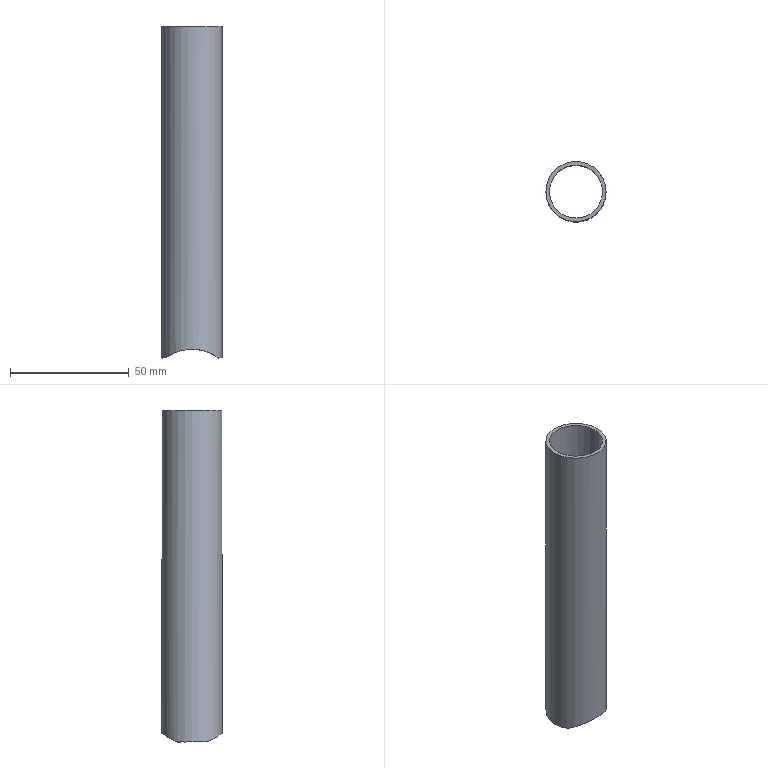Part | STEP file | 6151404 | 1 solid | 7 faces | box 25.4 x 25.4 x 140 mm | volume 15577 mm3 | cylinder 4 | plane 3 | commonest cylinder face diameters 38 x2 22.4 x1 25.4 x1
STEP:
#1=CARTESIAN_POINT('',(11.2,-5.987,-70.));
#2=VERTEX_POINT('',#1);
#3=CARTESIAN_POINT('',(11.2,5.987,-70.));
#4=VERTEX_POINT('',#3);
#5=CARTESIAN_POINT('',(0.,0.,-70.));
#6=DIRECTION('',(0.,0.,1.));
#7=DIRECTION('',(1.,0.,0.));
#8=AXIS2_PLACEMENT_3D('',#5,#6,#7);
#9=CIRCLE('',#8,12.7);
#10=EDGE_CURVE('',#2,#4,#9,.T.);
#11=ORIENTED_EDGE('',*,*,#10,.F.);
#12=CARTESIAN_POINT('',(11.2,0.,-70.));
#13=VERTEX_POINT('',#12);
#14=CARTESIAN_POINT('',(11.2,-30.,-70.));
#15=DIRECTION('',(0.,1.,0.));
#16=VECTOR('',#15,1000.);
#17=LINE('',#14,#16);
#18=EDGE_CURVE('',#2,#13,#17,.T.);
#19=ORIENTED_EDGE('',*,*,#18,.T.);
#20=CARTESIAN_POINT('',(11.2,-30.,-70.));
#21=DIRECTION('',(0.,1.,0.));
#22=VECTOR('',#21,1000.);
#23=LINE('',#20,#22);
#24=EDGE_CURVE('',#13,#4,#23,.T.);
#25=ORIENTED_EDGE('',*,*,#24,.T.);
#26=EDGE_LOOP('',(#11,#19,#25));
#27=FACE_OUTER_BOUND('',#26,.T.);
#28=CARTESIAN_POINT('',(0.,0.,-70.));
#29=DIRECTION('',(0.,0.,1.));
#30=DIRECTION('',(1.,0.,0.));
#31=AXIS2_PLACEMENT_3D('',#28,#29,#30);
#32=PLANE('',#31);
#33=ADVANCED_FACE('',(#27),#32,.F.);
#34=CARTESIAN_POINT('',(12.7,0.,70.));
#35=VERTEX_POINT('',#34);
#36=CARTESIAN_POINT('',(0.,0.,70.));
#37=DIRECTION('',(0.,0.,1.));
#38=DIRECTION('',(1.,0.,0.));
#39=AXIS2_PLACEMENT_3D('',#36,#37,#38);
#40=CIRCLE('',#39,12.7);
#41=EDGE_CURVE('',#35,#35,#40,.T.);
#42=ORIENTED_EDGE('',*,*,#41,.T.);
#43=EDGE_LOOP('',(#42));
#44=FACE_OUTER_BOUND('',#43,.T.);
#45=CARTESIAN_POINT('',(11.2,0.,70.));
#46=VERTEX_POINT('',#45);
#47=CARTESIAN_POINT('',(0.,0.,70.));
#48=DIRECTION('',(0.,0.,1.));
#49=DIRECTION('',(1.,0.,0.));
#50=AXIS2_PLACEMENT_3D('',#47,#48,#49);
#51=CIRCLE('',#50,11.2);
#52=EDGE_CURVE('',#46,#46,#51,.T.);
#53=ORIENTED_EDGE('',*,*,#52,.F.);
#54=EDGE_LOOP('',(#53));
#55=FACE_BOUND('',#54,.T.);
#56=CARTESIAN_POINT('',(0.,0.,70.));
#57=DIRECTION('',(0.,0.,1.));
#58=DIRECTION('',(1.,0.,0.));
#59=AXIS2_PLACEMENT_3D('',#56,#57,#58);
#60=PLANE('',#59);
#61=ADVANCED_FACE('',(#44,#55),#60,.T.);
#62=CARTESIAN_POINT('',(-11.2,5.987,-70.));
#63=VERTEX_POINT('',#62);
#64=CARTESIAN_POINT('',(-11.2,-5.987,-70.));
#65=VERTEX_POINT('',#64);
#66=CARTESIAN_POINT('',(0.,0.,-70.));
#67=DIRECTION('',(0.,0.,1.));
#68=DIRECTION('',(1.,0.,0.));
#69=AXIS2_PLACEMENT_3D('',#66,#67,#68);
#70=CIRCLE('',#69,12.7);
#71=EDGE_CURVE('',#63,#65,#70,.T.);
#72=ORIENTED_EDGE('',*,*,#71,.F.);
#73=CARTESIAN_POINT('',(-11.2,0.,-70.));
#74=VERTEX_POINT('',#73);
#75=CARTESIAN_POINT('',(-11.2,-30.,-70.));
#76=DIRECTION('',(0.,-1.,0.));
#77=VECTOR('',#76,1000.);
#78=LINE('',#75,#77);
#79=EDGE_CURVE('',#63,#74,#78,.T.);
#80=ORIENTED_EDGE('',*,*,#79,.T.);
#81=CARTESIAN_POINT('',(-11.2,-30.,-70.));
#82=DIRECTION('',(0.,-1.,0.));
#83=VECTOR('',#82,1000.);
#84=LINE('',#81,#83);
#85=EDGE_CURVE('',#74,#65,#84,.T.);
#86=ORIENTED_EDGE('',*,*,#85,.T.);
#87=EDGE_LOOP('',(#72,#80,#86));
#88=FACE_OUTER_BOUND('',#87,.T.);
#89=CARTESIAN_POINT('',(0.,0.,-70.));
#90=DIRECTION('',(0.,0.,1.));
#91=DIRECTION('',(1.,0.,0.));
#92=AXIS2_PLACEMENT_3D('',#89,#90,#91);
#93=PLANE('',#92);
#94=ADVANCED_FACE('',(#88),#93,.F.);
#95=ORIENTED_EDGE('',*,*,#41,.F.);
#96=EDGE_LOOP('',(#95));
#97=FACE_OUTER_BOUND('',#96,.T.);
#98=ORIENTED_EDGE('',*,*,#71,.T.);
#99=CARTESIAN_POINT('',(-11.2,-5.987,-70.));
#100=CARTESIAN_POINT('',(-10.665,-6.988,-69.61));
#101=CARTESIAN_POINT('',(-10.02,-7.882,-69.181));
#102=CARTESIAN_POINT('',(-9.072,-8.892,-68.652));
#103=CARTESIAN_POINT('',(-8.875,-9.088,-68.547));
#104=CARTESIAN_POINT('',(-8.467,-9.47,-68.337));
#105=CARTESIAN_POINT('',(-8.255,-9.655,-68.233));
#106=CARTESIAN_POINT('',(-7.604,-10.187,-67.929));
#107=CARTESIAN_POINT('',(-7.149,-10.512,-67.737));
#108=CARTESIAN_POINT('',(-6.192,-11.102,-67.378));
#109=CARTESIAN_POINT('',(-5.692,-11.368,-67.212));
#110=CARTESIAN_POINT('',(-4.639,-11.836,-66.915));
#111=CARTESIAN_POINT('',(-4.085,-12.039,-66.784));
#112=CARTESIAN_POINT('',(-2.962,-12.364,-66.572));
#113=CARTESIAN_POINT('',(-2.388,-12.487,-66.489));
#114=CARTESIAN_POINT('',(-1.215,-12.656,-66.378));
#115=CARTESIAN_POINT('',(-0.6122,-12.699,-66.349));
#116=CARTESIAN_POINT('',(0.5767,-12.701,-66.347));
#117=CARTESIAN_POINT('',(1.167,-12.66,-66.375));
#118=CARTESIAN_POINT('',(2.339,-12.497,-66.483));
#119=CARTESIAN_POINT('',(2.925,-12.373,-66.566));
#120=CARTESIAN_POINT('',(4.053,-12.05,-66.776));
#121=CARTESIAN_POINT('',(4.598,-11.853,-66.905));
#122=CARTESIAN_POINT('',(5.653,-11.387,-67.2));
#123=CARTESIAN_POINT('',(6.165,-11.118,-67.369));
#124=CARTESIAN_POINT('',(7.133,-10.523,-67.73));
#125=CARTESIAN_POINT('',(7.591,-10.197,-67.924));
#126=CARTESIAN_POINT('',(8.458,-9.49,-68.328));
#127=CARTESIAN_POINT('',(8.869,-9.107,-68.539));
#128=CARTESIAN_POINT('',(10.017,-7.887,-69.179));
#129=CARTESIAN_POINT('',(10.665,-6.988,-69.61));
#130=CARTESIAN_POINT('',(11.2,-5.987,-70.));
#131=B_SPLINE_CURVE_WITH_KNOTS('',3,(#99,#100,#101,#102,#103,#104,#105,#106,#107,#108,#109,#110,#111,#112,#113,#114,#115,#116,#117,#118,#119,#120,#121,#122,#123,#124,#125,#126,#127,#128,#129,#130),.UNSPECIFIED.,.F.,.F.,(4,2,2,2,2,2,2,2,2,2,2,2,2,2,2,4),(0.,0.003547,0.004433,0.00532,0.007093,0.008867,0.01064,0.01241,0.01419,0.01596,0.01773,0.01951,0.02128,0.02305,0.02483,0.02837),.UNSPECIFIED.);
#132=EDGE_CURVE('',#65,#2,#131,.T.);
#133=ORIENTED_EDGE('',*,*,#132,.T.);
#134=ORIENTED_EDGE('',*,*,#10,.T.);
#135=CARTESIAN_POINT('',(11.2,5.987,-70.));
#136=CARTESIAN_POINT('',(10.665,6.988,-69.61));
#137=CARTESIAN_POINT('',(10.02,7.882,-69.181));
#138=CARTESIAN_POINT('',(9.072,8.892,-68.652));
#139=CARTESIAN_POINT('',(8.875,9.088,-68.547));
#140=CARTESIAN_POINT('',(8.467,9.47,-68.337));
#141=CARTESIAN_POINT('',(8.255,9.655,-68.233));
#142=CARTESIAN_POINT('',(7.604,10.187,-67.929));
#143=CARTESIAN_POINT('',(7.149,10.512,-67.737));
#144=CARTESIAN_POINT('',(6.192,11.102,-67.378));
#145=CARTESIAN_POINT('',(5.692,11.368,-67.212));
#146=CARTESIAN_POINT('',(4.639,11.836,-66.915));
#147=CARTESIAN_POINT('',(4.085,12.039,-66.784));
#148=CARTESIAN_POINT('',(2.962,12.364,-66.572));
#149=CARTESIAN_POINT('',(2.388,12.487,-66.489));
#150=CARTESIAN_POINT('',(1.215,12.656,-66.378));
#151=CARTESIAN_POINT('',(0.6122,12.699,-66.349));
#152=CARTESIAN_POINT('',(-0.5767,12.701,-66.347));
#153=CARTESIAN_POINT('',(-1.167,12.66,-66.375));
#154=CARTESIAN_POINT('',(-2.339,12.497,-66.483));
#155=CARTESIAN_POINT('',(-2.925,12.373,-66.566));
#156=CARTESIAN_POINT('',(-4.053,12.05,-66.776));
#157=CARTESIAN_POINT('',(-4.598,11.853,-66.905));
#158=CARTESIAN_POINT('',(-5.653,11.387,-67.2));
#159=CARTESIAN_POINT('',(-6.165,11.118,-67.369));
#160=CARTESIAN_POINT('',(-7.133,10.523,-67.73));
#161=CARTESIAN_POINT('',(-7.591,10.197,-67.924));
#162=CARTESIAN_POINT('',(-8.458,9.49,-68.328));
#163=CARTESIAN_POINT('',(-8.869,9.107,-68.539));
#164=CARTESIAN_POINT('',(-10.017,7.887,-69.179));
#165=CARTESIAN_POINT('',(-10.665,6.988,-69.61));
#166=CARTESIAN_POINT('',(-11.2,5.987,-70.));
#167=B_SPLINE_CURVE_WITH_KNOTS('',3,(#135,#136,#137,#138,#139,#140,#141,#142,#143,#144,#145,#146,#147,#148,#149,#150,#151,#152,#153,#154,#155,#156,#157,#158,#159,#160,#161,#162,#163,#164,#165,#166),.UNSPECIFIED.,.F.,.F.,(4,2,2,2,2,2,2,2,2,2,2,2,2,2,2,4),(0.,0.003547,0.004433,0.00532,0.007093,0.008867,0.01064,0.01241,0.01419,0.01596,0.01773,0.01951,0.02128,0.02305,0.02483,0.02837),.UNSPECIFIED.);
#168=EDGE_CURVE('',#4,#63,#167,.T.);
#169=ORIENTED_EDGE('',*,*,#168,.T.);
#170=EDGE_LOOP('',(#98,#133,#134,#169));
#171=FACE_OUTER_BOUND('',#170,.T.);
#172=CARTESIAN_POINT('',(0.,0.,70.));
#173=DIRECTION('',(0.,0.,-1.));
#174=DIRECTION('',(-1.,0.,0.));
#175=AXIS2_PLACEMENT_3D('',#172,#173,#174);
#176=CYLINDRICAL_SURFACE('',#175,12.7);
#177=ADVANCED_FACE('',(#97,#171),#176,.T.);
#178=CARTESIAN_POINT('',(-11.2,0.,-70.));
#179=CARTESIAN_POINT('',(-11.2,-0.7603,-70.));
#180=CARTESIAN_POINT('',(-11.123,-1.503,-69.943));
#181=CARTESIAN_POINT('',(-10.828,-2.956,-69.734));
#182=CARTESIAN_POINT('',(-10.606,-3.673,-69.58));
#183=CARTESIAN_POINT('',(-10.04,-5.016,-69.214));
#184=CARTESIAN_POINT('',(-9.698,-5.65,-69.003));
#185=CARTESIAN_POINT('',(-8.89,-6.851,-68.55));
#186=CARTESIAN_POINT('',(-8.436,-7.401,-68.315));
#187=CARTESIAN_POINT('',(-7.681,-8.159,-67.968));
#188=CARTESIAN_POINT('',(-7.417,-8.4,-67.853));
#189=CARTESIAN_POINT('',(-6.862,-8.859,-67.628));
#190=CARTESIAN_POINT('',(-6.57,-9.077,-67.517));
#191=CARTESIAN_POINT('',(-5.674,-9.683,-67.204));
#192=CARTESIAN_POINT('',(-5.04,-10.029,-67.016));
#193=CARTESIAN_POINT('',(-4.03,-10.456,-66.777));
#194=CARTESIAN_POINT('',(-3.684,-10.584,-66.705));
#195=CARTESIAN_POINT('',(-2.969,-10.806,-66.578));
#196=CARTESIAN_POINT('',(-2.607,-10.899,-66.524));
#197=CARTESIAN_POINT('',(-1.514,-11.122,-66.394));
#198=CARTESIAN_POINT('',(-0.7732,-11.199,-66.349));
#199=CARTESIAN_POINT('',(0.3582,-11.201,-66.348));
#200=CARTESIAN_POINT('',(0.7396,-11.182,-66.359));
#201=CARTESIAN_POINT('',(1.488,-11.107,-66.403));
#202=CARTESIAN_POINT('',(1.857,-11.051,-66.435));
#203=CARTESIAN_POINT('',(2.587,-10.903,-66.521));
#204=CARTESIAN_POINT('',(2.947,-10.812,-66.574));
#205=CARTESIAN_POINT('',(3.66,-10.592,-66.7));
#206=CARTESIAN_POINT('',(4.011,-10.464,-66.773));
#207=CARTESIAN_POINT('',(5.029,-10.035,-67.012));
#208=CARTESIAN_POINT('',(5.667,-9.688,-67.202));
#209=CARTESIAN_POINT('',(6.57,-9.078,-67.517));
#210=CARTESIAN_POINT('',(6.861,-8.86,-67.628));
#211=CARTESIAN_POINT('',(7.415,-8.401,-67.852));
#212=CARTESIAN_POINT('',(7.679,-8.161,-67.967));
#213=CARTESIAN_POINT('',(8.183,-7.655,-68.198));
#214=CARTESIAN_POINT('',(8.423,-7.391,-68.315));
#215=CARTESIAN_POINT('',(8.878,-6.837,-68.548));
#216=CARTESIAN_POINT('',(9.095,-6.546,-68.664));
#217=CARTESIAN_POINT('',(9.697,-5.65,-69.002));
#218=CARTESIAN_POINT('',(10.039,-5.019,-69.213));
#219=CARTESIAN_POINT('',(10.461,-4.017,-69.486));
#220=CARTESIAN_POINT('',(10.587,-3.673,-69.57));
#221=CARTESIAN_POINT('',(10.807,-2.965,-69.72));
#222=CARTESIAN_POINT('',(10.9,-2.601,-69.785));
#223=CARTESIAN_POINT('',(11.123,-1.505,-69.943));
#224=CARTESIAN_POINT('',(11.2,-0.7604,-70.));
#225=CARTESIAN_POINT('',(11.2,0.,-70.));
#226=B_SPLINE_CURVE_WITH_KNOTS('',3,(#178,#179,#180,#181,#182,#183,#184,#185,#186,#187,#188,#189,#190,#191,#192,#193,#194,#195,#196,#197,#198,#199,#200,#201,#202,#203,#204,#205,#206,#207,#208,#209,#210,#211,#212,#213,#214,#215,#216,#217,#218,#219,#220,#221,#222,#223,#224,#225),.UNSPECIFIED.,.F.,.F.,(4,2,2,2,2,2,2,2,2,2,2,2,2,2,2,2,2,2,2,2,2,2,2,4),(0.,0.002243,0.004485,0.006728,0.00897,0.01009,0.01121,0.01346,0.01458,0.0157,0.01794,0.01906,0.02018,0.0213,0.02243,0.02467,0.02579,0.02691,0.02803,0.02915,0.0314,0.03252,0.03364,0.03588),.UNSPECIFIED.);
#227=EDGE_CURVE('',#74,#13,#226,.T.);
#228=ORIENTED_EDGE('',*,*,#227,.F.);
#229=CARTESIAN_POINT('',(11.2,0.,-70.));
#230=CARTESIAN_POINT('',(11.2,0.759,-70.));
#231=CARTESIAN_POINT('',(11.123,1.505,-69.943));
#232=CARTESIAN_POINT('',(10.901,2.597,-69.786));
#233=CARTESIAN_POINT('',(10.808,2.959,-69.721));
#234=CARTESIAN_POINT('',(10.589,3.668,-69.572));
#235=CARTESIAN_POINT('',(10.463,4.013,-69.487));
#236=CARTESIAN_POINT('',(10.18,4.684,-69.304));
#237=CARTESIAN_POINT('',(10.023,5.011,-69.205));
#238=CARTESIAN_POINT('',(9.679,5.648,-68.997));
#239=CARTESIAN_POINT('',(9.49,5.959,-68.886));
#240=CARTESIAN_POINT('',(8.886,6.855,-68.548));
#241=CARTESIAN_POINT('',(8.433,7.405,-68.313));
#242=CARTESIAN_POINT('',(7.424,8.416,-67.85));
#243=CARTESIAN_POINT('',(6.863,8.88,-67.619));
#244=CARTESIAN_POINT('',(5.671,9.685,-67.203));
#245=CARTESIAN_POINT('',(5.037,10.03,-67.015));
#246=CARTESIAN_POINT('',(4.023,10.459,-66.775));
#247=CARTESIAN_POINT('',(3.671,10.588,-66.703));
#248=CARTESIAN_POINT('',(2.961,10.808,-66.577));
#249=CARTESIAN_POINT('',(2.601,10.9,-66.523));
#250=CARTESIAN_POINT('',(1.512,11.122,-66.394));
#251=CARTESIAN_POINT('',(0.7696,11.199,-66.348));
#252=CARTESIAN_POINT('',(-0.7494,11.201,-66.348));
#253=CARTESIAN_POINT('',(-1.496,11.125,-66.393));
#254=CARTESIAN_POINT('',(-2.957,10.828,-66.565));
#255=CARTESIAN_POINT('',(-3.678,10.604,-66.694));
#256=CARTESIAN_POINT('',(-5.032,10.033,-67.013));
#257=CARTESIAN_POINT('',(-5.672,9.685,-67.203));
#258=CARTESIAN_POINT('',(-6.879,8.868,-67.625));
#259=CARTESIAN_POINT('',(-7.43,8.411,-67.852));
#260=CARTESIAN_POINT('',(-8.186,7.652,-68.2));
#261=CARTESIAN_POINT('',(-8.427,7.387,-68.317));
#262=CARTESIAN_POINT('',(-8.883,6.831,-68.551));
#263=CARTESIAN_POINT('',(-9.099,6.541,-68.667));
#264=CARTESIAN_POINT('',(-9.698,5.648,-69.003));
#265=CARTESIAN_POINT('',(-10.04,5.017,-69.214));
#266=CARTESIAN_POINT('',(-10.463,4.011,-69.488));
#267=CARTESIAN_POINT('',(-10.59,3.664,-69.573));
#268=CARTESIAN_POINT('',(-10.81,2.954,-69.722));
#269=CARTESIAN_POINT('',(-10.902,2.594,-69.786));
#270=CARTESIAN_POINT('',(-11.049,1.868,-69.891));
#271=CARTESIAN_POINT('',(-11.105,1.5,-69.931));
#272=CARTESIAN_POINT('',(-11.181,0.7569,-69.986));
#273=CARTESIAN_POINT('',(-11.2,0.3794,-70.));
#274=CARTESIAN_POINT('',(-11.2,0.,-70.));
#275=B_SPLINE_CURVE_WITH_KNOTS('',3,(#229,#230,#231,#232,#233,#234,#235,#236,#237,#238,#239,#240,#241,#242,#243,#244,#245,#246,#247,#248,#249,#250,#251,#252,#253,#254,#255,#256,#257,#258,#259,#260,#261,#262,#263,#264,#265,#266,#267,#268,#269,#270,#271,#272,#273,#274),.UNSPECIFIED.,.F.,.F.,(4,2,2,2,2,2,2,2,2,2,2,2,2,2,2,2,2,2,2,2,2,2,4),(0.03588,0.03812,0.03924,0.04036,0.04148,0.0426,0.04484,0.04707,0.04931,0.05043,0.05155,0.05379,0.05603,0.05827,0.0605,0.06274,0.06386,0.06498,0.06722,0.06834,0.06946,0.07058,0.0717),.UNSPECIFIED.);
#276=EDGE_CURVE('',#13,#74,#275,.T.);
#277=ORIENTED_EDGE('',*,*,#276,.F.);
#278=EDGE_LOOP('',(#228,#277));
#279=FACE_OUTER_BOUND('',#278,.T.);
#280=ORIENTED_EDGE('',*,*,#52,.T.);
#281=EDGE_LOOP('',(#280));
#282=FACE_OUTER_BOUND('',#281,.T.);
#283=CARTESIAN_POINT('',(0.,0.,70.));
#284=DIRECTION('',(0.,0.,-1.));
#285=DIRECTION('',(-1.,0.,0.));
#286=AXIS2_PLACEMENT_3D('',#283,#284,#285);
#287=CYLINDRICAL_SURFACE('',#286,11.2);
#288=ADVANCED_FACE('',(#279,#282),#287,.F.);
#289=ORIENTED_EDGE('',*,*,#168,.F.);
#290=ORIENTED_EDGE('',*,*,#24,.F.);
#291=ORIENTED_EDGE('',*,*,#276,.T.);
#292=ORIENTED_EDGE('',*,*,#79,.F.);
#293=EDGE_LOOP('',(#289,#290,#291,#292));
#294=FACE_OUTER_BOUND('',#293,.T.);
#295=CARTESIAN_POINT('',(0.,-30.,-85.348));
#296=DIRECTION('',(0.,1.,0.));
#297=DIRECTION('',(0.,0.,1.));
#298=AXIS2_PLACEMENT_3D('',#295,#296,#297);
#299=CYLINDRICAL_SURFACE('',#298,19.);
#300=ADVANCED_FACE('',(#294),#299,.F.);
#301=ORIENTED_EDGE('',*,*,#132,.F.);
#302=ORIENTED_EDGE('',*,*,#85,.F.);
#303=ORIENTED_EDGE('',*,*,#227,.T.);
#304=ORIENTED_EDGE('',*,*,#18,.F.);
#305=EDGE_LOOP('',(#301,#302,#303,#304));
#306=FACE_OUTER_BOUND('',#305,.T.);
#307=CARTESIAN_POINT('',(0.,-30.,-85.348));
#308=DIRECTION('',(0.,1.,0.));
#309=DIRECTION('',(0.,0.,1.));
#310=AXIS2_PLACEMENT_3D('',#307,#308,#309);
#311=CYLINDRICAL_SURFACE('',#310,19.);
#312=ADVANCED_FACE('',(#306),#311,.F.);
#313=CLOSED_SHELL('',(#33,#61,#94,#177,#288,#300,#312));
#314=MANIFOLD_SOLID_BREP('',#313);
#315=CARTESIAN_POINT('',(0.,0.,0.));
#316=DIRECTION('',(0.,0.,1.));
#317=DIRECTION('',(1.,0.,0.));
#318=AXIS2_PLACEMENT_3D('',#315,#316,#317);
#319=(LENGTH_UNIT()NAMED_UNIT(*)SI_UNIT(.MILLI.,.METRE.));
#320=UNCERTAINTY_MEASURE_WITH_UNIT(LENGTH_MEASURE(0.00001),#319,'','');
#321=(NAMED_UNIT(*)PLANE_ANGLE_UNIT()SI_UNIT($,.RADIAN.));
#322=(NAMED_UNIT(*)SI_UNIT($,.STERADIAN.)SOLID_ANGLE_UNIT());
#323=(GEOMETRIC_REPRESENTATION_CONTEXT(3)GLOBAL_UNCERTAINTY_ASSIGNED_CONTEXT((#320))GLOBAL_UNIT_ASSIGNED_CONTEXT((#319,#321,#322))REPRESENTATION_CONTEXT('',''));
#324=ADVANCED_BREP_SHAPE_REPRESENTATION('',(#314,#318),#323);